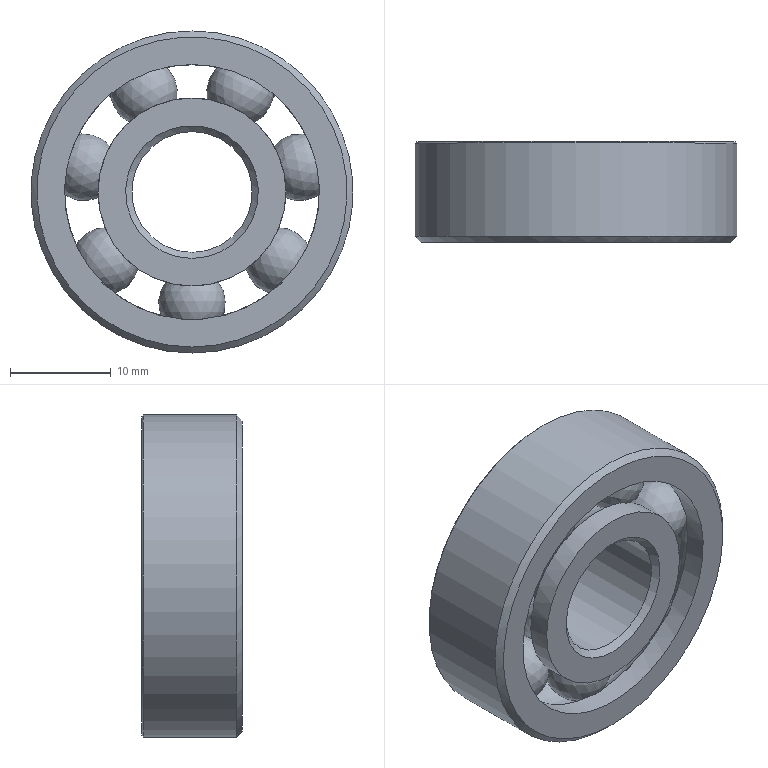Part | STEP file | YBQDJ-DX-6 | 1 solid | 35 faces | box 32 x 10 x 32 mm | volume 4745 mm3 | torus 14 | sphere 7 | cylinder 5 | cone 5 | plane 4 | commonest cylinder face diameters 18.667 x2 12 x1 25.333 x1 32 x1